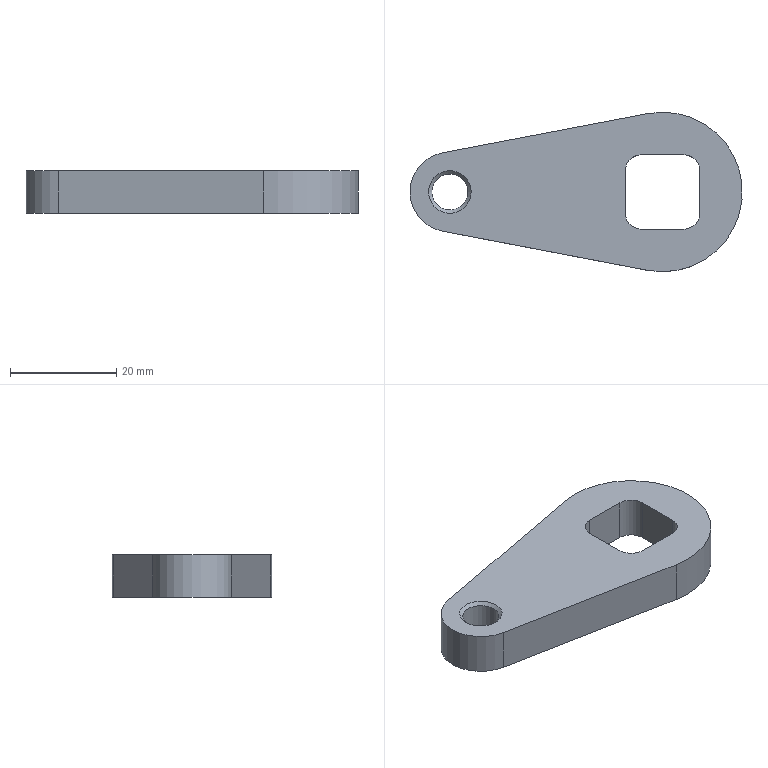Part | NX | features DATUM_CSYS 2, BLEND 1, EXTRUDE 1, HOLE PACKAGE 1, SIMPLE HOLE 1, SKETCH 1, SYMBOLIC_THREAD 1 | 1 solid | 17 faces | box 62.5 x 30 x 8 mm | volume 9056 mm3 | plane 8 | cylinder 7 | cone 2 | commonest cylinder face diameters 6 x4 6.8 x1 15 x1 30 x1
STEP:
#1=CARTESIAN_POINT('',(33.,-4.,-4.));
#2=VERTEX_POINT('',#1);
#3=CARTESIAN_POINT('',(33.,4.,-4.));
#4=VERTEX_POINT('',#3);
#5=CARTESIAN_POINT('',(33.,-7.,-4.));
#6=DIRECTION('',(0.,1.,0.));
#7=VECTOR('',#6,1000.);
#8=LINE('',#5,#7);
#9=EDGE_CURVE('',#2,#4,#8,.T.);
#10=ORIENTED_EDGE('',*,*,#9,.T.);
#11=CARTESIAN_POINT('',(33.,4.,4.));
#12=VERTEX_POINT('',#11);
#13=CARTESIAN_POINT('',(33.,4.,4.));
#14=DIRECTION('',(0.,0.,-1.));
#15=VECTOR('',#14,1000.);
#16=LINE('',#13,#15);
#17=EDGE_CURVE('',#4,#12,#16,.F.);
#18=ORIENTED_EDGE('',*,*,#17,.T.);
#19=CARTESIAN_POINT('',(33.,-4.,4.));
#20=VERTEX_POINT('',#19);
#21=CARTESIAN_POINT('',(33.,-7.,4.));
#22=DIRECTION('',(0.,1.,0.));
#23=VECTOR('',#22,1000.);
#24=LINE('',#21,#23);
#25=EDGE_CURVE('',#20,#12,#24,.T.);
#26=ORIENTED_EDGE('',*,*,#25,.F.);
#27=CARTESIAN_POINT('',(33.,-4.,-4.));
#28=DIRECTION('',(0.,0.,-1.));
#29=VECTOR('',#28,1000.);
#30=LINE('',#27,#29);
#31=EDGE_CURVE('',#20,#2,#30,.T.);
#32=ORIENTED_EDGE('',*,*,#31,.T.);
#33=EDGE_LOOP('',(#10,#18,#26,#32));
#34=FACE_BOUND('',#33,.T.);
#35=CARTESIAN_POINT('',(33.,-7.,4.));
#36=DIRECTION('',(-1.,0.,0.));
#37=DIRECTION('',(0.,0.,1.));
#38=AXIS2_PLACEMENT_3D('',#35,#36,#37);
#39=PLANE('',#38);
#40=ADVANCED_FACE('',(#34),#39,.F.);
#41=CARTESIAN_POINT('',(36.,7.,-4.));
#42=VERTEX_POINT('',#41);
#43=CARTESIAN_POINT('',(44.,7.,-4.));
#44=VERTEX_POINT('',#43);
#45=CARTESIAN_POINT('',(33.,7.,-4.));
#46=DIRECTION('',(1.,0.,0.));
#47=VECTOR('',#46,1000.);
#48=LINE('',#45,#47);
#49=EDGE_CURVE('',#42,#44,#48,.T.);
#50=ORIENTED_EDGE('',*,*,#49,.T.);
#51=CARTESIAN_POINT('',(44.,7.,4.));
#52=VERTEX_POINT('',#51);
#53=CARTESIAN_POINT('',(44.,7.,4.));
#54=DIRECTION('',(0.,0.,-1.));
#55=VECTOR('',#54,1000.);
#56=LINE('',#53,#55);
#57=EDGE_CURVE('',#44,#52,#56,.F.);
#58=ORIENTED_EDGE('',*,*,#57,.T.);
#59=CARTESIAN_POINT('',(36.,7.,4.));
#60=VERTEX_POINT('',#59);
#61=CARTESIAN_POINT('',(33.,7.,4.));
#62=DIRECTION('',(1.,0.,0.));
#63=VECTOR('',#62,1000.);
#64=LINE('',#61,#63);
#65=EDGE_CURVE('',#60,#52,#64,.T.);
#66=ORIENTED_EDGE('',*,*,#65,.F.);
#67=CARTESIAN_POINT('',(36.,7.,-4.));
#68=DIRECTION('',(0.,0.,-1.));
#69=VECTOR('',#68,1000.);
#70=LINE('',#67,#69);
#71=EDGE_CURVE('',#60,#42,#70,.T.);
#72=ORIENTED_EDGE('',*,*,#71,.T.);
#73=EDGE_LOOP('',(#50,#58,#66,#72));
#74=FACE_BOUND('',#73,.T.);
#75=CARTESIAN_POINT('',(33.,7.,4.));
#76=DIRECTION('',(0.,1.,0.));
#77=DIRECTION('',(-1.,0.,0.));
#78=AXIS2_PLACEMENT_3D('',#75,#76,#77);
#79=PLANE('',#78);
#80=ADVANCED_FACE('',(#74),#79,.F.);
#81=CARTESIAN_POINT('',(47.,4.,4.));
#82=VERTEX_POINT('',#81);
#83=CARTESIAN_POINT('',(47.,-4.,4.));
#84=VERTEX_POINT('',#83);
#85=CARTESIAN_POINT('',(47.,7.,4.));
#86=DIRECTION('',(0.,-1.,0.));
#87=VECTOR('',#86,1000.);
#88=LINE('',#85,#87);
#89=EDGE_CURVE('',#82,#84,#88,.T.);
#90=ORIENTED_EDGE('',*,*,#89,.F.);
#91=CARTESIAN_POINT('',(47.,4.,-4.));
#92=VERTEX_POINT('',#91);
#93=CARTESIAN_POINT('',(47.,4.,-4.));
#94=DIRECTION('',(0.,0.,-1.));
#95=VECTOR('',#94,1000.);
#96=LINE('',#93,#95);
#97=EDGE_CURVE('',#82,#92,#96,.T.);
#98=ORIENTED_EDGE('',*,*,#97,.T.);
#99=CARTESIAN_POINT('',(47.,-4.,-4.));
#100=VERTEX_POINT('',#99);
#101=CARTESIAN_POINT('',(47.,7.,-4.));
#102=DIRECTION('',(0.,-1.,0.));
#103=VECTOR('',#102,1000.);
#104=LINE('',#101,#103);
#105=EDGE_CURVE('',#92,#100,#104,.T.);
#106=ORIENTED_EDGE('',*,*,#105,.T.);
#107=CARTESIAN_POINT('',(47.,-4.,4.));
#108=DIRECTION('',(0.,0.,-1.));
#109=VECTOR('',#108,1000.);
#110=LINE('',#107,#109);
#111=EDGE_CURVE('',#100,#84,#110,.F.);
#112=ORIENTED_EDGE('',*,*,#111,.T.);
#113=EDGE_LOOP('',(#90,#98,#106,#112));
#114=FACE_BOUND('',#113,.T.);
#115=CARTESIAN_POINT('',(47.,7.,4.));
#116=DIRECTION('',(1.,0.,0.));
#117=DIRECTION('',(0.,0.,-1.));
#118=AXIS2_PLACEMENT_3D('',#115,#116,#117);
#119=PLANE('',#118);
#120=ADVANCED_FACE('',(#114),#119,.F.);
#121=CARTESIAN_POINT('',(-1.406,7.367,-4.));
#122=VERTEX_POINT('',#121);
#123=CARTESIAN_POINT('',(-1.406,-7.367,-4.));
#124=VERTEX_POINT('',#123);
#125=CARTESIAN_POINT('',(0.,0.,-4.));
#126=DIRECTION('',(0.,0.,1.));
#127=DIRECTION('',(1.,0.,0.));
#128=AXIS2_PLACEMENT_3D('',#125,#126,#127);
#129=CIRCLE('',#128,7.5);
#130=EDGE_CURVE('',#122,#124,#129,.T.);
#131=ORIENTED_EDGE('',*,*,#130,.T.);
#132=CARTESIAN_POINT('',(-1.406,-7.367,4.));
#133=VERTEX_POINT('',#132);
#134=CARTESIAN_POINT('',(-1.406,-7.367,4.));
#135=DIRECTION('',(0.,0.,-1.));
#136=VECTOR('',#135,1000.);
#137=LINE('',#134,#136);
#138=EDGE_CURVE('',#133,#124,#137,.T.);
#139=ORIENTED_EDGE('',*,*,#138,.F.);
#140=CARTESIAN_POINT('',(-1.406,7.367,4.));
#141=VERTEX_POINT('',#140);
#142=CARTESIAN_POINT('',(0.,0.,4.));
#143=DIRECTION('',(0.,0.,1.));
#144=DIRECTION('',(1.,0.,0.));
#145=AXIS2_PLACEMENT_3D('',#142,#143,#144);
#146=CIRCLE('',#145,7.5);
#147=EDGE_CURVE('',#141,#133,#146,.T.);
#148=ORIENTED_EDGE('',*,*,#147,.F.);
#149=CARTESIAN_POINT('',(-1.406,7.367,4.));
#150=DIRECTION('',(0.,0.,-1.));
#151=VECTOR('',#150,1000.);
#152=LINE('',#149,#151);
#153=EDGE_CURVE('',#141,#122,#152,.T.);
#154=ORIENTED_EDGE('',*,*,#153,.T.);
#155=EDGE_LOOP('',(#131,#139,#148,#154));
#156=FACE_BOUND('',#155,.T.);
#157=CARTESIAN_POINT('',(0.,0.,4.));
#158=DIRECTION('',(0.,0.,-1.));
#159=DIRECTION('',(-1.,0.,0.));
#160=AXIS2_PLACEMENT_3D('',#157,#158,#159);
#161=CYLINDRICAL_SURFACE('',#160,7.5);
#162=ADVANCED_FACE('',(#156),#161,.T.);
#163=CARTESIAN_POINT('',(37.187,-14.734,-4.));
#164=VERTEX_POINT('',#163);
#165=CARTESIAN_POINT('',(-1.406,-7.367,-4.));
#166=DIRECTION('',(0.9823,-0.1875,0.));
#167=VECTOR('',#166,1000.);
#168=LINE('',#165,#167);
#169=EDGE_CURVE('',#124,#164,#168,.T.);
#170=ORIENTED_EDGE('',*,*,#169,.T.);
#171=CARTESIAN_POINT('',(37.187,-14.734,4.));
#172=VERTEX_POINT('',#171);
#173=CARTESIAN_POINT('',(37.187,-14.734,4.));
#174=DIRECTION('',(0.,0.,-1.));
#175=VECTOR('',#174,1000.);
#176=LINE('',#173,#175);
#177=EDGE_CURVE('',#172,#164,#176,.T.);
#178=ORIENTED_EDGE('',*,*,#177,.F.);
#179=CARTESIAN_POINT('',(-1.406,-7.367,4.));
#180=DIRECTION('',(0.9823,-0.1875,0.));
#181=VECTOR('',#180,1000.);
#182=LINE('',#179,#181);
#183=EDGE_CURVE('',#133,#172,#182,.T.);
#184=ORIENTED_EDGE('',*,*,#183,.F.);
#185=ORIENTED_EDGE('',*,*,#138,.T.);
#186=EDGE_LOOP('',(#170,#178,#184,#185));
#187=FACE_BOUND('',#186,.T.);
#188=CARTESIAN_POINT('',(-1.406,-7.367,4.));
#189=DIRECTION('',(0.1875,0.9823,0.));
#190=DIRECTION('',(-0.9823,0.1875,0.));
#191=AXIS2_PLACEMENT_3D('',#188,#189,#190);
#192=PLANE('',#191);
#193=ADVANCED_FACE('',(#187),#192,.F.);
#194=CARTESIAN_POINT('',(37.187,14.734,-4.));
#195=VERTEX_POINT('',#194);
#196=CARTESIAN_POINT('',(40.,0.,-4.));
#197=DIRECTION('',(0.,0.,1.));
#198=DIRECTION('',(1.,0.,0.));
#199=AXIS2_PLACEMENT_3D('',#196,#197,#198);
#200=CIRCLE('',#199,15.);
#201=EDGE_CURVE('',#164,#195,#200,.T.);
#202=ORIENTED_EDGE('',*,*,#201,.T.);
#203=CARTESIAN_POINT('',(37.187,14.734,4.));
#204=VERTEX_POINT('',#203);
#205=CARTESIAN_POINT('',(37.187,14.734,4.));
#206=DIRECTION('',(0.,0.,-1.));
#207=VECTOR('',#206,1000.);
#208=LINE('',#205,#207);
#209=EDGE_CURVE('',#204,#195,#208,.T.);
#210=ORIENTED_EDGE('',*,*,#209,.F.);
#211=CARTESIAN_POINT('',(40.,0.,4.));
#212=DIRECTION('',(0.,0.,1.));
#213=DIRECTION('',(1.,0.,0.));
#214=AXIS2_PLACEMENT_3D('',#211,#212,#213);
#215=CIRCLE('',#214,15.);
#216=EDGE_CURVE('',#172,#204,#215,.T.);
#217=ORIENTED_EDGE('',*,*,#216,.F.);
#218=ORIENTED_EDGE('',*,*,#177,.T.);
#219=EDGE_LOOP('',(#202,#210,#217,#218));
#220=FACE_BOUND('',#219,.T.);
#221=CARTESIAN_POINT('',(40.,0.,4.));
#222=DIRECTION('',(0.,0.,-1.));
#223=DIRECTION('',(-1.,0.,0.));
#224=AXIS2_PLACEMENT_3D('',#221,#222,#223);
#225=CYLINDRICAL_SURFACE('',#224,15.);
#226=ADVANCED_FACE('',(#220),#225,.T.);
#227=CARTESIAN_POINT('',(37.187,14.734,-4.));
#228=DIRECTION('',(-0.9823,-0.1875,0.));
#229=VECTOR('',#228,1000.);
#230=LINE('',#227,#229);
#231=EDGE_CURVE('',#195,#122,#230,.T.);
#232=ORIENTED_EDGE('',*,*,#231,.T.);
#233=ORIENTED_EDGE('',*,*,#153,.F.);
#234=CARTESIAN_POINT('',(37.187,14.734,4.));
#235=DIRECTION('',(-0.9823,-0.1875,0.));
#236=VECTOR('',#235,1000.);
#237=LINE('',#234,#236);
#238=EDGE_CURVE('',#204,#141,#237,.T.);
#239=ORIENTED_EDGE('',*,*,#238,.F.);
#240=ORIENTED_EDGE('',*,*,#209,.T.);
#241=EDGE_LOOP('',(#232,#233,#239,#240));
#242=FACE_BOUND('',#241,.T.);
#243=CARTESIAN_POINT('',(37.187,14.734,4.));
#244=DIRECTION('',(0.1875,-0.9823,0.));
#245=DIRECTION('',(0.9823,0.1875,0.));
#246=AXIS2_PLACEMENT_3D('',#243,#244,#245);
#247=PLANE('',#246);
#248=ADVANCED_FACE('',(#242),#247,.F.);
#249=CARTESIAN_POINT('',(44.,-7.,-4.));
#250=VERTEX_POINT('',#249);
#251=CARTESIAN_POINT('',(36.,-7.,-4.));
#252=VERTEX_POINT('',#251);
#253=CARTESIAN_POINT('',(47.,-7.,-4.));
#254=DIRECTION('',(-1.,0.,0.));
#255=VECTOR('',#254,1000.);
#256=LINE('',#253,#255);
#257=EDGE_CURVE('',#250,#252,#256,.T.);
#258=ORIENTED_EDGE('',*,*,#257,.T.);
#259=CARTESIAN_POINT('',(36.,-7.,4.));
#260=VERTEX_POINT('',#259);
#261=CARTESIAN_POINT('',(36.,-7.,4.));
#262=DIRECTION('',(0.,0.,-1.));
#263=VECTOR('',#262,1000.);
#264=LINE('',#261,#263);
#265=EDGE_CURVE('',#252,#260,#264,.F.);
#266=ORIENTED_EDGE('',*,*,#265,.T.);
#267=CARTESIAN_POINT('',(44.,-7.,4.));
#268=VERTEX_POINT('',#267);
#269=CARTESIAN_POINT('',(47.,-7.,4.));
#270=DIRECTION('',(-1.,0.,0.));
#271=VECTOR('',#270,1000.);
#272=LINE('',#269,#271);
#273=EDGE_CURVE('',#268,#260,#272,.T.);
#274=ORIENTED_EDGE('',*,*,#273,.F.);
#275=CARTESIAN_POINT('',(44.,-7.,-4.));
#276=DIRECTION('',(0.,0.,-1.));
#277=VECTOR('',#276,1000.);
#278=LINE('',#275,#277);
#279=EDGE_CURVE('',#268,#250,#278,.T.);
#280=ORIENTED_EDGE('',*,*,#279,.T.);
#281=EDGE_LOOP('',(#258,#266,#274,#280));
#282=FACE_BOUND('',#281,.T.);
#283=CARTESIAN_POINT('',(47.,-7.,4.));
#284=DIRECTION('',(0.,-1.,0.));
#285=DIRECTION('',(1.,0.,0.));
#286=AXIS2_PLACEMENT_3D('',#283,#284,#285);
#287=PLANE('',#286);
#288=ADVANCED_FACE('',(#282),#287,.F.);
#289=CARTESIAN_POINT('',(4.,0.,4.));
#290=VERTEX_POINT('',#289);
#291=CARTESIAN_POINT('',(0.,0.,4.));
#292=DIRECTION('',(0.,0.,1.));
#293=DIRECTION('',(1.,0.,0.));
#294=AXIS2_PLACEMENT_3D('',#291,#292,#293);
#295=CIRCLE('',#294,4.);
#296=EDGE_CURVE('',#290,#290,#295,.F.);
#297=ORIENTED_EDGE('',*,*,#296,.T.);
#298=EDGE_LOOP('',(#297));
#299=FACE_BOUND('',#298,.T.);
#300=ORIENTED_EDGE('',*,*,#147,.T.);
#301=ORIENTED_EDGE('',*,*,#183,.T.);
#302=ORIENTED_EDGE('',*,*,#216,.T.);
#303=ORIENTED_EDGE('',*,*,#238,.T.);
#304=EDGE_LOOP('',(#300,#301,#302,#303));
#305=FACE_BOUND('',#304,.T.);
#306=ORIENTED_EDGE('',*,*,#273,.T.);
#307=CARTESIAN_POINT('',(36.,-4.,4.));
#308=DIRECTION('',(0.,0.,1.));
#309=DIRECTION('',(1.,0.,0.));
#310=AXIS2_PLACEMENT_3D('',#307,#308,#309);
#311=CIRCLE('',#310,3.);
#312=EDGE_CURVE('',#260,#20,#311,.F.);
#313=ORIENTED_EDGE('',*,*,#312,.T.);
#314=ORIENTED_EDGE('',*,*,#25,.T.);
#315=CARTESIAN_POINT('',(36.,4.,4.));
#316=DIRECTION('',(0.,0.,1.));
#317=DIRECTION('',(1.,0.,0.));
#318=AXIS2_PLACEMENT_3D('',#315,#316,#317);
#319=CIRCLE('',#318,3.);
#320=EDGE_CURVE('',#12,#60,#319,.F.);
#321=ORIENTED_EDGE('',*,*,#320,.T.);
#322=ORIENTED_EDGE('',*,*,#65,.T.);
#323=CARTESIAN_POINT('',(44.,4.,4.));
#324=DIRECTION('',(0.,0.,1.));
#325=DIRECTION('',(1.,0.,0.));
#326=AXIS2_PLACEMENT_3D('',#323,#324,#325);
#327=CIRCLE('',#326,3.);
#328=EDGE_CURVE('',#52,#82,#327,.F.);
#329=ORIENTED_EDGE('',*,*,#328,.T.);
#330=ORIENTED_EDGE('',*,*,#89,.T.);
#331=CARTESIAN_POINT('',(44.,-4.,4.));
#332=DIRECTION('',(0.,0.,1.));
#333=DIRECTION('',(1.,0.,0.));
#334=AXIS2_PLACEMENT_3D('',#331,#332,#333);
#335=CIRCLE('',#334,3.);
#336=EDGE_CURVE('',#84,#268,#335,.F.);
#337=ORIENTED_EDGE('',*,*,#336,.T.);
#338=EDGE_LOOP('',(#306,#313,#314,#321,#322,#329,#330,#337));
#339=FACE_BOUND('',#338,.T.);
#340=CARTESIAN_POINT('',(0.,0.,4.));
#341=DIRECTION('',(0.,0.,1.));
#342=DIRECTION('',(1.,0.,0.));
#343=AXIS2_PLACEMENT_3D('',#340,#341,#342);
#344=PLANE('',#343);
#345=ADVANCED_FACE('',(#299,#305,#339),#344,.T.);
#346=CARTESIAN_POINT('',(4.,0.,-4.));
#347=VERTEX_POINT('',#346);
#348=CARTESIAN_POINT('',(0.,0.,-4.));
#349=DIRECTION('',(0.,0.,1.));
#350=DIRECTION('',(1.,0.,0.));
#351=AXIS2_PLACEMENT_3D('',#348,#349,#350);
#352=CIRCLE('',#351,4.);
#353=EDGE_CURVE('',#347,#347,#352,.T.);
#354=ORIENTED_EDGE('',*,*,#353,.T.);
#355=EDGE_LOOP('',(#354));
#356=FACE_BOUND('',#355,.T.);
#357=ORIENTED_EDGE('',*,*,#130,.F.);
#358=ORIENTED_EDGE('',*,*,#231,.F.);
#359=ORIENTED_EDGE('',*,*,#201,.F.);
#360=ORIENTED_EDGE('',*,*,#169,.F.);
#361=EDGE_LOOP('',(#357,#358,#359,#360));
#362=FACE_BOUND('',#361,.T.);
#363=ORIENTED_EDGE('',*,*,#9,.F.);
#364=CARTESIAN_POINT('',(36.,-4.,-4.));
#365=DIRECTION('',(0.,0.,1.));
#366=DIRECTION('',(1.,0.,0.));
#367=AXIS2_PLACEMENT_3D('',#364,#365,#366);
#368=CIRCLE('',#367,3.);
#369=EDGE_CURVE('',#2,#252,#368,.T.);
#370=ORIENTED_EDGE('',*,*,#369,.T.);
#371=ORIENTED_EDGE('',*,*,#257,.F.);
#372=CARTESIAN_POINT('',(44.,-4.,-4.));
#373=DIRECTION('',(0.,0.,1.));
#374=DIRECTION('',(1.,0.,0.));
#375=AXIS2_PLACEMENT_3D('',#372,#373,#374);
#376=CIRCLE('',#375,3.);
#377=EDGE_CURVE('',#250,#100,#376,.T.);
#378=ORIENTED_EDGE('',*,*,#377,.T.);
#379=ORIENTED_EDGE('',*,*,#105,.F.);
#380=CARTESIAN_POINT('',(44.,4.,-4.));
#381=DIRECTION('',(0.,0.,1.));
#382=DIRECTION('',(1.,0.,0.));
#383=AXIS2_PLACEMENT_3D('',#380,#381,#382);
#384=CIRCLE('',#383,3.);
#385=EDGE_CURVE('',#92,#44,#384,.T.);
#386=ORIENTED_EDGE('',*,*,#385,.T.);
#387=ORIENTED_EDGE('',*,*,#49,.F.);
#388=CARTESIAN_POINT('',(36.,4.,-4.));
#389=DIRECTION('',(0.,0.,1.));
#390=DIRECTION('',(1.,0.,0.));
#391=AXIS2_PLACEMENT_3D('',#388,#389,#390);
#392=CIRCLE('',#391,3.);
#393=EDGE_CURVE('',#42,#4,#392,.T.);
#394=ORIENTED_EDGE('',*,*,#393,.T.);
#395=EDGE_LOOP('',(#363,#370,#371,#378,#379,#386,#387,#394));
#396=FACE_BOUND('',#395,.T.);
#397=CARTESIAN_POINT('',(0.,0.,-4.));
#398=DIRECTION('',(0.,0.,1.));
#399=DIRECTION('',(1.,0.,0.));
#400=AXIS2_PLACEMENT_3D('',#397,#398,#399);
#401=PLANE('',#400);
#402=ADVANCED_FACE('',(#356,#362,#396),#401,.F.);
#403=CARTESIAN_POINT('',(3.4,0.,-3.4));
#404=VERTEX_POINT('',#403);
#405=CARTESIAN_POINT('',(0.,0.,-3.4));
#406=DIRECTION('',(0.,0.,1.));
#407=DIRECTION('',(1.,0.,0.));
#408=AXIS2_PLACEMENT_3D('',#405,#406,#407);
#409=CIRCLE('',#408,3.4);
#410=EDGE_CURVE('',#404,#404,#409,.F.);
#411=ORIENTED_EDGE('',*,*,#410,.T.);
#412=EDGE_LOOP('',(#411));
#413=FACE_BOUND('',#412,.T.);
#414=CARTESIAN_POINT('',(3.4,0.,3.4));
#415=VERTEX_POINT('',#414);
#416=CARTESIAN_POINT('',(0.,0.,3.4));
#417=DIRECTION('',(0.,0.,1.));
#418=DIRECTION('',(1.,0.,0.));
#419=AXIS2_PLACEMENT_3D('',#416,#417,#418);
#420=CIRCLE('',#419,3.4);
#421=EDGE_CURVE('',#415,#415,#420,.T.);
#422=ORIENTED_EDGE('',*,*,#421,.T.);
#423=EDGE_LOOP('',(#422));
#424=FACE_BOUND('',#423,.T.);
#425=CARTESIAN_POINT('',(0.,0.,4.));
#426=DIRECTION('',(0.,0.,-1.));
#427=DIRECTION('',(-1.,0.,0.));
#428=AXIS2_PLACEMENT_3D('',#425,#426,#427);
#429=CYLINDRICAL_SURFACE('',#428,3.4);
#430=ADVANCED_FACE('',(#413,#424),#429,.F.);
#431=ORIENTED_EDGE('',*,*,#421,.F.);
#432=EDGE_LOOP('',(#431));
#433=FACE_BOUND('',#432,.T.);
#434=ORIENTED_EDGE('',*,*,#296,.F.);
#435=EDGE_LOOP('',(#434));
#436=FACE_BOUND('',#435,.T.);
#437=CARTESIAN_POINT('',(0.,0.,4.));
#438=DIRECTION('',(0.,0.,1.));
#439=DIRECTION('',(1.,0.,0.));
#440=AXIS2_PLACEMENT_3D('',#437,#438,#439);
#441=CONICAL_SURFACE('',#440,4.,0.7854);
#442=ADVANCED_FACE('',(#433,#436),#441,.F.);
#443=ORIENTED_EDGE('',*,*,#410,.F.);
#444=EDGE_LOOP('',(#443));
#445=FACE_BOUND('',#444,.T.);
#446=ORIENTED_EDGE('',*,*,#353,.F.);
#447=EDGE_LOOP('',(#446));
#448=FACE_BOUND('',#447,.T.);
#449=CARTESIAN_POINT('',(0.,0.,-4.));
#450=DIRECTION('',(0.,0.,-1.));
#451=DIRECTION('',(-1.,0.,0.));
#452=AXIS2_PLACEMENT_3D('',#449,#450,#451);
#453=CONICAL_SURFACE('',#452,4.,0.7854);
#454=ADVANCED_FACE('',(#445,#448),#453,.F.);
#455=ORIENTED_EDGE('',*,*,#328,.F.);
#456=ORIENTED_EDGE('',*,*,#57,.F.);
#457=ORIENTED_EDGE('',*,*,#385,.F.);
#458=ORIENTED_EDGE('',*,*,#97,.F.);
#459=EDGE_LOOP('',(#455,#456,#457,#458));
#460=FACE_BOUND('',#459,.T.);
#461=CARTESIAN_POINT('',(44.,4.,4.));
#462=DIRECTION('',(0.,0.,1.));
#463=DIRECTION('',(1.,0.,0.));
#464=AXIS2_PLACEMENT_3D('',#461,#462,#463);
#465=CYLINDRICAL_SURFACE('',#464,3.);
#466=ADVANCED_FACE('',(#460),#465,.F.);
#467=ORIENTED_EDGE('',*,*,#320,.F.);
#468=ORIENTED_EDGE('',*,*,#17,.F.);
#469=ORIENTED_EDGE('',*,*,#393,.F.);
#470=ORIENTED_EDGE('',*,*,#71,.F.);
#471=EDGE_LOOP('',(#467,#468,#469,#470));
#472=FACE_BOUND('',#471,.T.);
#473=CARTESIAN_POINT('',(36.,4.,4.));
#474=DIRECTION('',(0.,0.,1.));
#475=DIRECTION('',(1.,0.,0.));
#476=AXIS2_PLACEMENT_3D('',#473,#474,#475);
#477=CYLINDRICAL_SURFACE('',#476,3.);
#478=ADVANCED_FACE('',(#472),#477,.F.);
#479=ORIENTED_EDGE('',*,*,#312,.F.);
#480=ORIENTED_EDGE('',*,*,#265,.F.);
#481=ORIENTED_EDGE('',*,*,#369,.F.);
#482=ORIENTED_EDGE('',*,*,#31,.F.);
#483=EDGE_LOOP('',(#479,#480,#481,#482));
#484=FACE_BOUND('',#483,.T.);
#485=CARTESIAN_POINT('',(36.,-4.,4.));
#486=DIRECTION('',(0.,0.,1.));
#487=DIRECTION('',(1.,0.,0.));
#488=AXIS2_PLACEMENT_3D('',#485,#486,#487);
#489=CYLINDRICAL_SURFACE('',#488,3.);
#490=ADVANCED_FACE('',(#484),#489,.F.);
#491=ORIENTED_EDGE('',*,*,#336,.F.);
#492=ORIENTED_EDGE('',*,*,#111,.F.);
#493=ORIENTED_EDGE('',*,*,#377,.F.);
#494=ORIENTED_EDGE('',*,*,#279,.F.);
#495=EDGE_LOOP('',(#491,#492,#493,#494));
#496=FACE_BOUND('',#495,.T.);
#497=CARTESIAN_POINT('',(44.,-4.,4.));
#498=DIRECTION('',(0.,0.,1.));
#499=DIRECTION('',(1.,0.,0.));
#500=AXIS2_PLACEMENT_3D('',#497,#498,#499);
#501=CYLINDRICAL_SURFACE('',#500,3.);
#502=ADVANCED_FACE('',(#496),#501,.F.);
#503=CLOSED_SHELL('',(#40,#80,#120,#162,#193,#226,#248,#288,#345,#402,#430,#442,#454,#466,#478,#490,#502));
#504=MANIFOLD_SOLID_BREP('',#503);
#505=(LENGTH_UNIT()NAMED_UNIT(*)SI_UNIT(.MILLI.,.METRE.));
#506=UNCERTAINTY_MEASURE_WITH_UNIT(LENGTH_MEASURE(0.00001),#505,'','');
#507=(NAMED_UNIT(*)PLANE_ANGLE_UNIT()SI_UNIT($,.RADIAN.));
#508=(NAMED_UNIT(*)SI_UNIT($,.STERADIAN.)SOLID_ANGLE_UNIT());
#509=(GEOMETRIC_REPRESENTATION_CONTEXT(3)GLOBAL_UNCERTAINTY_ASSIGNED_CONTEXT((#506))GLOBAL_UNIT_ASSIGNED_CONTEXT((#505,#507,#508))REPRESENTATION_CONTEXT('',''));
#510=ADVANCED_BREP_SHAPE_REPRESENTATION('',(#504),#509);